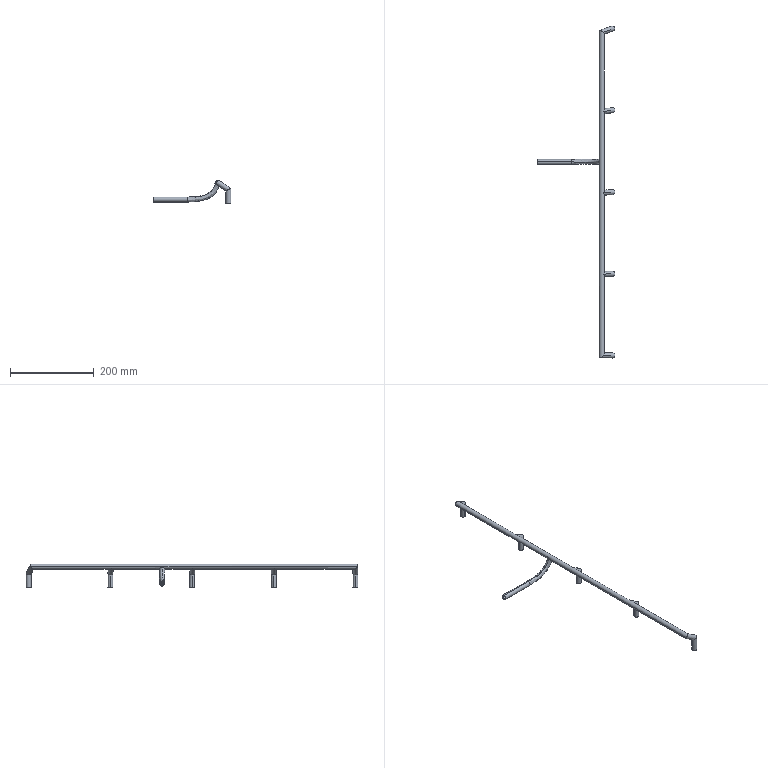Part | SolidWorks | features Sweep 5, 3DProfileFeature 2 | 1 solid | 97 faces | box 185.606 x 792 x 56.756 mm | volume 78943 mm3 | cylinder 74 | plane 14 | spline 9 | commonest cylinder face diameters 8 x37 12 x37